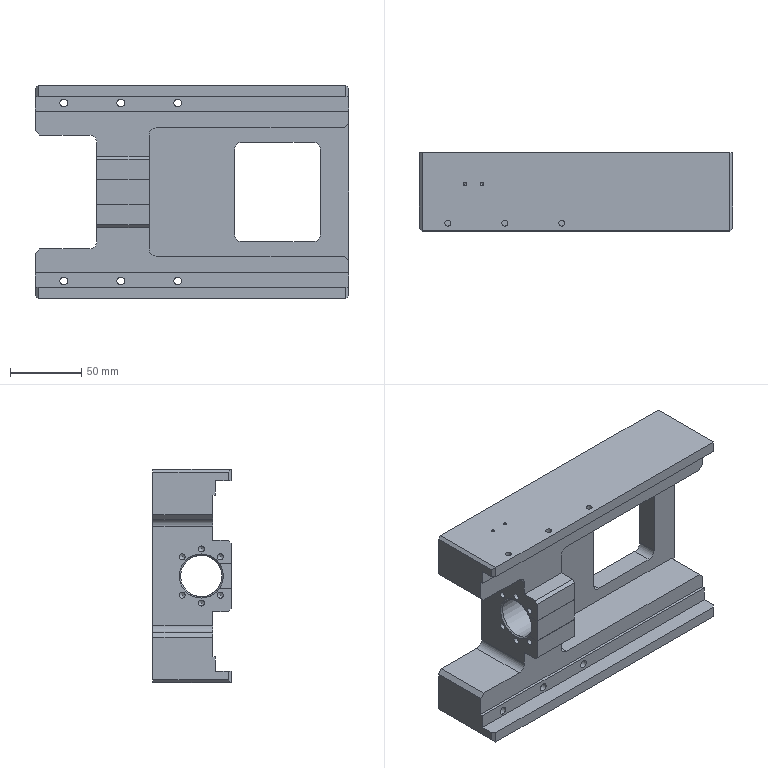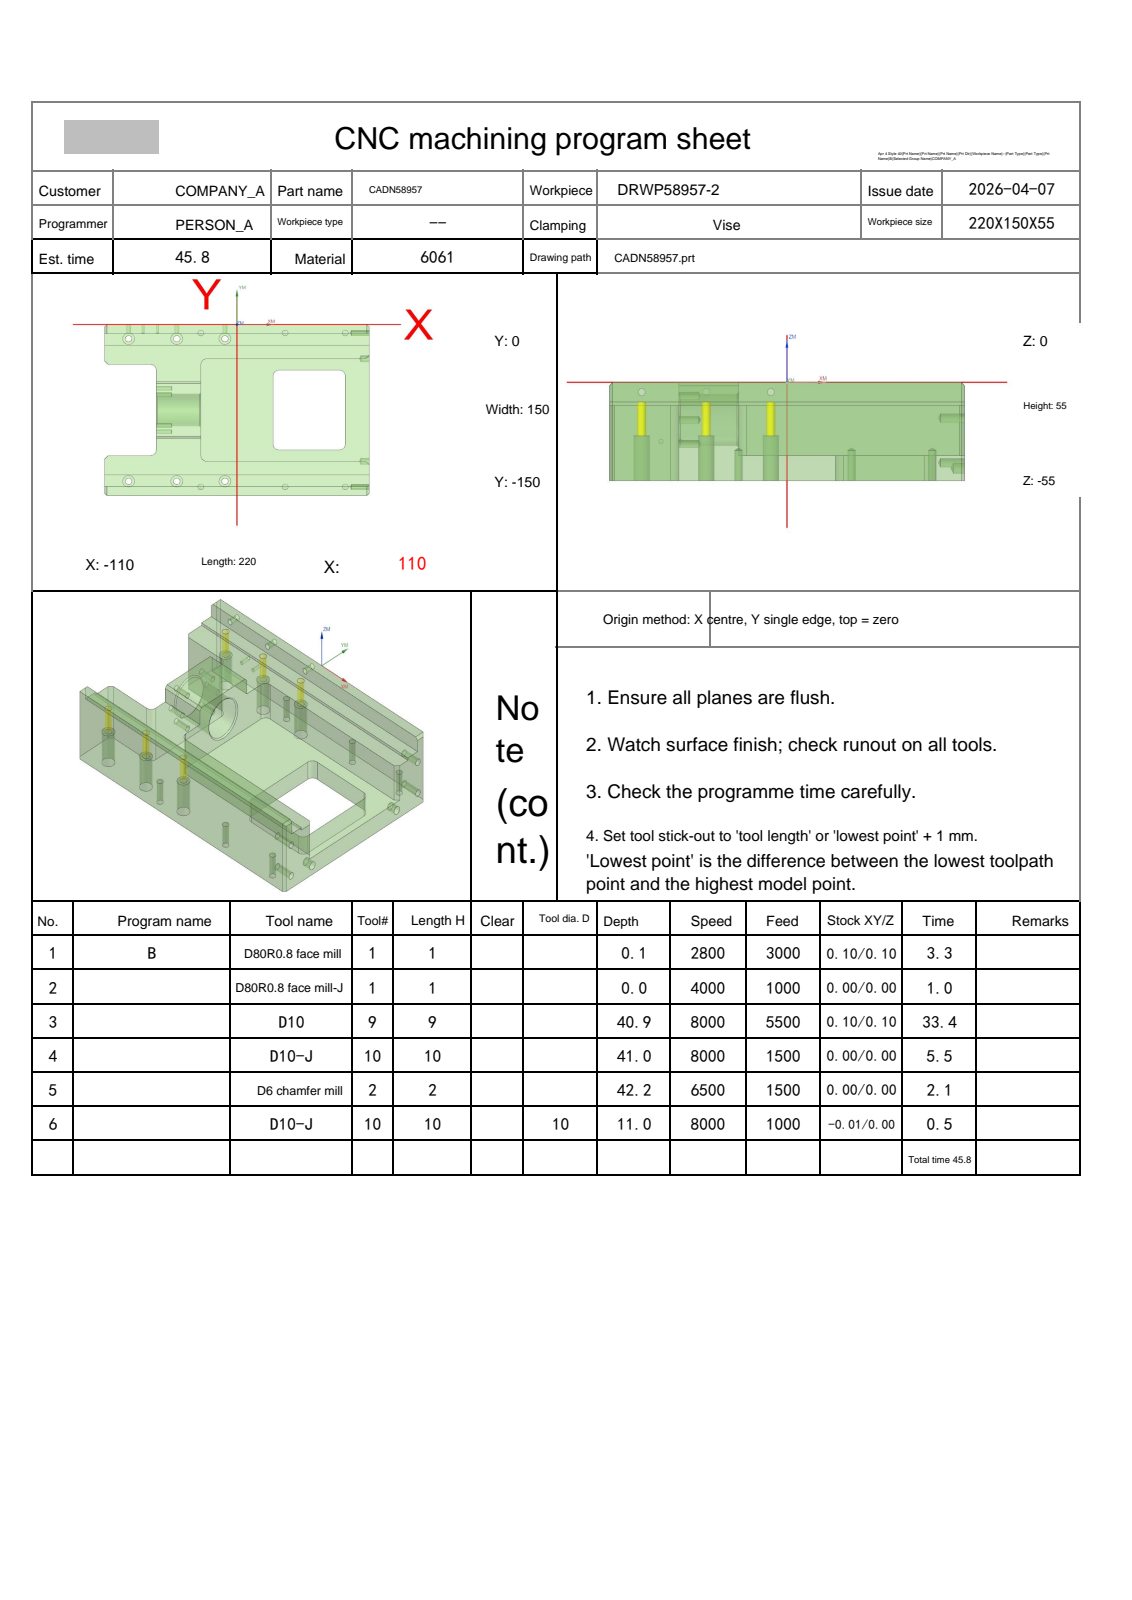NC program | NX | posted by the shop | part box 220 x 55 x 150 mm
Lines 1 to 208 of 15484:
%
O0001
(Machine time: 46.76 MIN)
(===Total Tool:4===)
(T1=D80R0.8 face mill D=80.  R=0.8  D-  H01 Z=0.    )
(T9=D10     D=10.  R=0.   D-  H09 Z=-40.9 )
(T10=D10-J  D=10.  R=0.   D10 H10 Z=-41.  )
(T2=D6 chamfer mill   D=6.   R=0.   D-  H02 Z=-42.2 )
G80 G90 G17 G49 G40
G91 G28 Z0
M01
N1 T01 M06
(D80R0.8 face mill  D=80. R=0.8 H=01 ce=0.10 di=0.10)
G00 G90 G54 X162.097 Y-126.097 M03 S2800
G43 H01 Z20.
M08
Z6.011
G01 Z4.011 F3000.
X150.097
X-142.1
G02 X-150.097 Y-118.1 I.003 J8.
G01 Y-104.704
G02 X-147.755 Y-99.049 I8. J-.001
G01 X-129.727 Y-81.021
G02 X-124.075 Y-78.68 I5.655 J-5.659
G01 X142.897
G03 X150.097 Y-71.48 I0.0 J7.2
G01 Y-39.263
G03 X142.097 Y-31.263 I-8. J0.0
G01 X-150.097
X-162.097
Z6.011
G00 X162.097 Y-126.097
Z5.522
G01 Z3.522
X150.097
X-142.1
G02 X-150.097 Y-118.1 I.003 J8.
G01 Y-104.704
G02 X-147.755 Y-99.049 I8. J-.001
G01 X-129.727 Y-81.021
G02 X-124.075 Y-78.68 I5.655 J-5.659
G01 X142.897
G03 X150.097 Y-71.48 I0.0 J7.2
G01 Y-39.263
G03 X142.097 Y-31.263 I-8. J0.0
G01 X-150.097
X-162.097
Z5.522
G00 X162.097 Y-126.097
Z5.033
G01 Z3.033
X150.097
X-142.1
G02 X-150.097 Y-118.1 I.003 J8.
G01 Y-104.704
G02 X-147.755 Y-99.049 I8. J-.001
G01 X-129.727 Y-81.021
G02 X-124.075 Y-78.68 I5.655 J-5.659
G01 X142.897
G03 X150.097 Y-71.48 I0.0 J7.2
G01 Y-39.263
G03 X142.097 Y-31.263 I-8. J0.0
G01 X-150.097
X-162.097
Z5.033
G00 X162.097 Y-126.097
Z4.544
G01 Z2.544
X150.097
X-142.1
G02 X-150.097 Y-118.1 I.003 J8.
G01 Y-104.704
G02 X-147.755 Y-99.049 I8. J-.001
G01 X-129.727 Y-81.021
G02 X-124.075 Y-78.68 I5.655 J-5.659
G01 X142.897
G03 X150.097 Y-71.48 I0.0 J7.2
G01 Y-39.263
G03 X142.097 Y-31.263 I-8. J0.0
G01 X-150.097
X-162.097
Z4.544
G00 Z20.
X162.097 Y-126.097
Z4.056
G01 Z2.056
X150.097
X-142.1
G02 X-150.097 Y-118.1 I.003 J8.
G01 Y-104.704
G02 X-147.755 Y-99.049 I8. J-.001
G01 X-129.727 Y-81.021
G02 X-124.075 Y-78.68 I5.655 J-5.659
G01 X142.897
G03 X150.097 Y-71.48 I0.0 J7.2
G01 Y-39.263
G03 X142.097 Y-31.263 I-8. J0.0
G01 X-150.097
X-162.097
Z4.056
G00 Z20.
X162.097 Y-126.097
Z3.567
G01 Z1.567
X150.097
X-142.1
G02 X-150.097 Y-118.1 I.003 J8.
G01 Y-104.704
G02 X-147.755 Y-99.049 I8. J-.001
G01 X-129.727 Y-81.021
G02 X-124.075 Y-78.68 I5.655 J-5.659
G01 X142.897
G03 X150.097 Y-71.48 I0.0 J7.2
G01 Y-39.263
G03 X142.097 Y-31.263 I-8. J0.0
G01 X-150.097
X-162.097
Z3.567
G00 Z20.
X162.097 Y-126.097
Z3.078
G01 Z1.078
X150.097
X-142.1
G02 X-150.097 Y-118.1 I.003 J8.
G01 Y-104.704
G02 X-147.755 Y-99.049 I8. J-.001
G01 X-129.727 Y-81.021
G02 X-124.075 Y-78.68 I5.655 J-5.659
G01 X142.897
G03 X150.097 Y-71.48 I0.0 J7.2
G01 Y-39.263
G03 X142.097 Y-31.263 I-8. J0.0
G01 X-150.097
X-162.097
Z3.078
G00 Z20.
X162.097 Y-126.097
Z2.589
G01 Z.589
X150.097
X-142.1
G02 X-150.097 Y-118.1 I.003 J8.
G01 Y-104.704
G02 X-147.755 Y-99.049 I8. J-.001
G01 X-129.727 Y-81.021
G02 X-124.075 Y-78.68 I5.655 J-5.659
G01 X142.897
G03 X150.097 Y-71.48 I0.0 J7.2
G01 Y-39.263
G03 X142.097 Y-31.263 I-8. J0.0
G01 X-150.097
X-162.097
Z2.589
G00 Z20.
X162.097 Y-126.097
Z2.1
G01 Z.1
X150.097
X-142.1
G02 X-150.097 Y-118.1 I.003 J8.
G01 Y-104.704
G02 X-147.755 Y-99.049 I8. J-.001
G01 X-129.727 Y-81.021
G02 X-124.075 Y-78.68 I5.655 J-5.659
G01 X142.897
G03 X150.097 Y-71.48 I0.0 J7.2
G01 Y-39.263
G03 X142.097 Y-31.263 I-8. J0.0
G01 X-150.097
X-162.097
Z2.1
G00 Z20.
G91 G28 Z0.0
M05
M09
G91 G28 Z0.0
M01
N2 T01 M06
(D80R0.8 face mill-J  D=80. R=0.8 H=01 ce=0.00 di=0.00)
G00 G90 G54 X161.999 Y-125.999 M03 S4000
G43 H01 Z20.
M08
Z2.
G01 Z0.0 F1000.
X149.999
X-142.002
G02 X-149.999 Y-118.002 I.003 J8.
G01 Y-104.744
G02 X-147.657 Y-99.09 I8. J-.001
G01 X-129.588 Y-81.021
G02 X-123.937 Y-78.68 I5.655 J-5.659
G01 X142.799
G03 X149.999 Y-71.48 I0.0 J7.2
G01 Y-39.361
G03 X141.999 Y-31.361 I-8. J0.0
G01 X-149.999
X-161.999
Z2.
G00 Z20.
G91 G28 Z0.0
M05
M09
G91 G28 Z0.0
M01